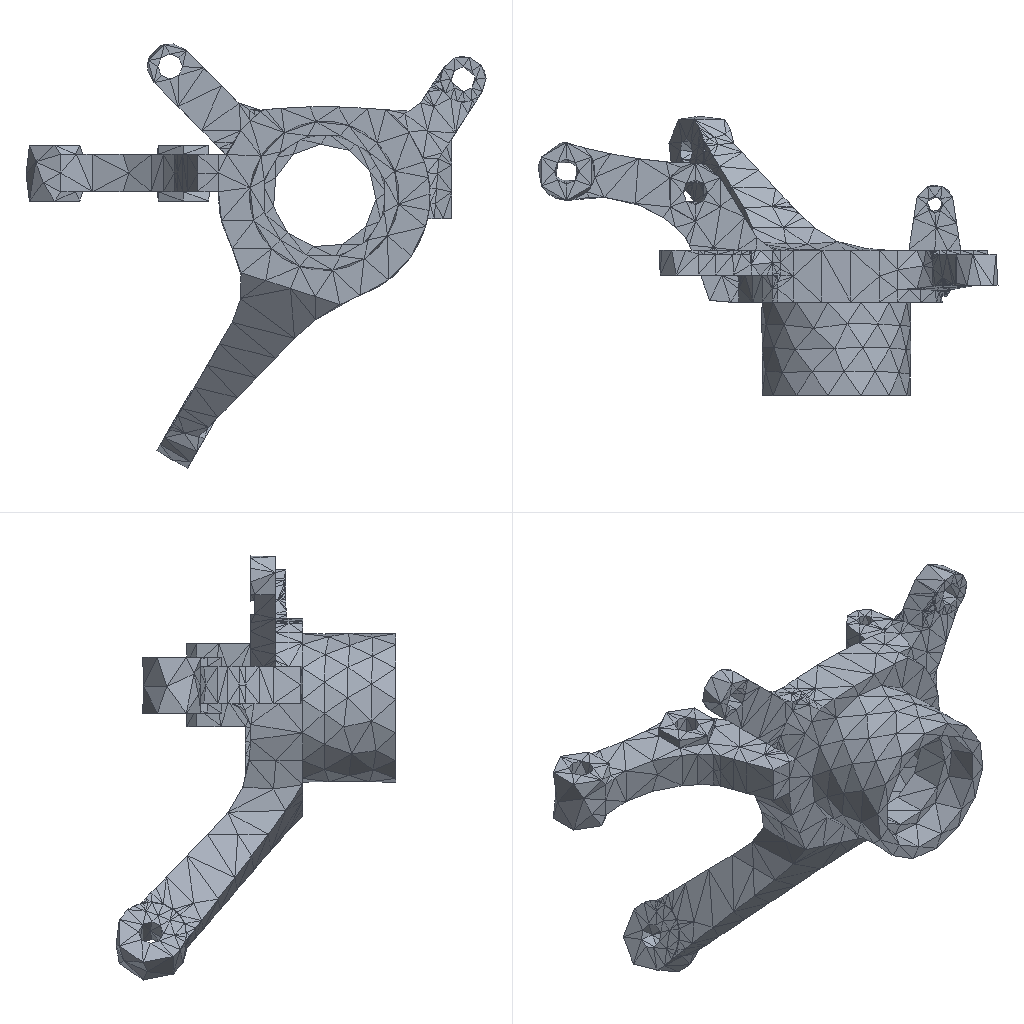Simulation study | ansys workbench
Set-up summary:
category,name,step,type,value,unit,region
solver,ansys_mapdl
solver,version,,,22.1
solver,version,,,22.1
units,MPA,,stated
analysis,deck1,,transient,transient
load_step,requested,,,1
analysis,nlgeom,,,True
mesh,nodes,,,5989
mesh,elements,,,3414
element_type,ANSYS 187 (type 1),,solid,2979
element_type,ANSYS 154 (type 2),,surface,435
load,load commands in deck,,count,3
bc,support commands in deck,,count,1
named_set,_FIXEDSU,,component
analysis,deck2,,transient,transient
load_step,requested,,,1
analysis,nlgeom,,,True
mesh,nodes,,,5989
mesh,elements,,,3427
element_type,ANSYS 187 (type 1),,solid,2979
element_type,ANSYS 154 (type 2),,surface,448
load,load commands in deck,,count,3
bc,support commands in deck,,count,1
named_set,_FIXEDSU,,component
material,1,,in results
material,1,,in results
check,setup vs results,,match,435 surface effect element(s) are not in the reader's mesh and were not compared
check,setup vs results,,match,448 surface effect element(s) are not in the reader's mesh and were not compared
Results summary:
result,analysis,,,static
result,last_loadstep,,,1
result,primary field,,,displacement
result,reaction total,1,FX,-35354.611,N
result,reaction total,1,FY,5.2e-05,N
result,reaction total,1,FZ,35354.611,N
result,mass,,,0.002973,"NMM: mm, ton, N, s, mV, mA, degC"
result,analysis,,,static
result,last_loadstep,,,1
result,primary field,,,displacement
result,reaction total,1,FX,0.0,N
result,reaction total,1,FY,51995.706,N
result,reaction total,1,FZ,9e-06,N
result,mass,,,0.002973,"NMM: mm, ton, N, s, mV, mA, degC"